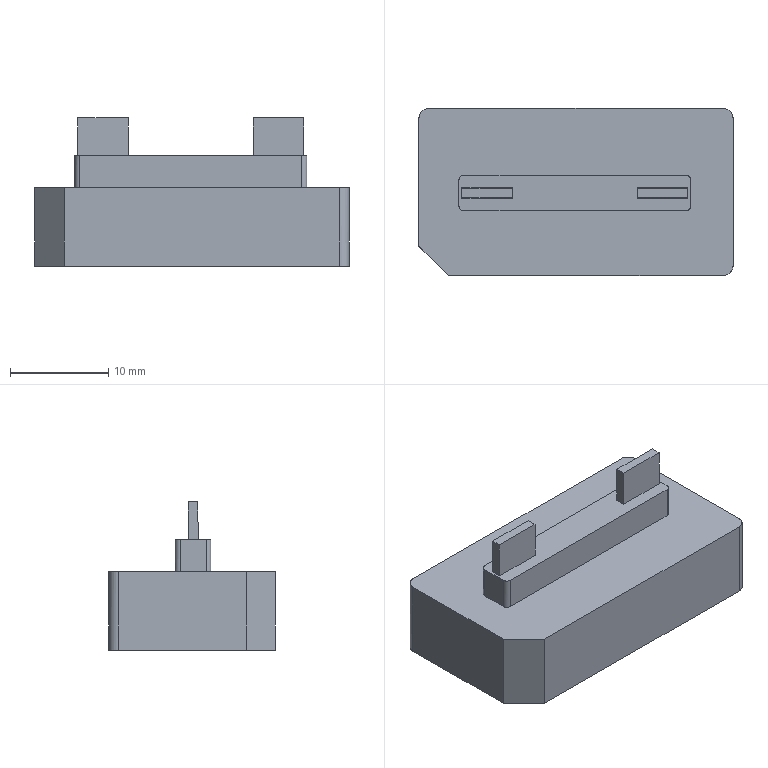NC program | PowerMill | posted by the shop | part box 32 x 17 x 15.109 mm
Lines 3100 to 3995 of 56729:
( TOOL ID   D10_1_1 )
( TOOL DIA. 10. TIP RAD 0 LENGTH 70.28 )
( Z = -4.119 )
T3 M6
T10
G91 G28 Z0
G0 G90 G54
M08
S8500 M3
X0 Y0 M8
G43 Z11.799 H3
X13.266 Y12.165
Z-2.919
G1 Z-4.119 F360
X12.287 Y6.982 F600
X9.889 Y5.783
X11.383
X11.664 Y5.776
G2 X12.775 Y5.6 I-.312 J-5.563
G1 X13.045 Y5.52
X13.311 Y5.426
G2 X14.073 Y5.062 I-2.083 J-5.347
X14.545 Y4.755 I-3.25 J-5.522
G1 X14.768 Y4.584
X14.983 Y4.401
X15.187 Y4.207
X15.381 Y4.003
G2 X15.735 Y3.565 I-4.735 J-4.197
G1 X15.895 Y3.333
X16.042 Y3.093
X16.176 Y2.845
X16.297 Y2.591
X16.405 Y2.331
X16.499 Y2.065
X16.579 Y1.795
X16.645 Y1.521
X16.696 Y1.245
X16.733 Y.965
X16.755 Y.684
X16.763 Y.403
Y-.627
X16.755 Y-.909
X16.733 Y-1.189
X16.696 Y-1.469
X16.645 Y-1.746
X16.579 Y-2.019
X16.499 Y-2.29
X16.405 Y-2.555
X16.297 Y-2.815
X16.176 Y-3.07
X16.042 Y-3.317
G2 X15.735 Y-3.789 I-5.478 J3.222
X15.381 Y-4.227 I-5.136 J3.797
G1 X15.187 Y-4.431
X14.983 Y-4.625
X14.768 Y-4.808
G2 X14.313 Y-5.139 I-3.867 J4.843
X13.825 Y-5.421 I-3.471 J5.449
X13.311 Y-5.65 I-2.868 J5.75
X12.775 Y-5.824 I-2.247 J6.004
X12.224 Y-5.941 I-1.618 J6.257
X11.664 Y-6. I-.95 J6.341
G1 X11.383 Y-6.007
X6.223
X6.042 Y-6.003
X5.661 Y-5.978
G2 X4.56 Y-5.744 I.603 J5.54
G1 X4.294 Y-5.649
X4.035 Y-5.542
G2 X3.293 Y-5.139 I2.352 J5.216
X2.837 Y-4.808 I3.524 J5.329
G1 X2.623 Y-4.625
X2.419 Y-4.431
X2.225 Y-4.227
X2.042 Y-4.013
X1.871 Y-3.789
X1.712 Y-3.558
X1.564 Y-3.317
X1.429 Y-3.07
X1.308 Y-2.815
X1.2 Y-2.555
X1.106 Y-2.29
X1.026 Y-2.019
X.961 Y-1.746
X.909 Y-1.469
X.872 Y-1.189
X.85 Y-.909
X.843 Y-.627
Y.403
X.85 Y.684
X.872 Y.965
X.909 Y1.245
X.961 Y1.521
X1.026 Y1.795
X1.106 Y2.065
X1.2 Y2.331
X1.308 Y2.591
X1.429 Y2.845
X1.564 Y3.093
X1.712 Y3.335
X1.871 Y3.565
G2 X2.196 Y3.969 I4.542 J-3.328
G1 X2.419 Y4.207
X2.623 Y4.401
G2 X3.061 Y4.755 I4.088 J-4.601
X3.533 Y5.062 I3.742 J-5.244
X4.035 Y5.318 I3.159 J-5.579
G1 X4.294 Y5.425
X4.56 Y5.52
G2 X5.104 Y5.665 I1.94 J-6.152
X5.661 Y5.753 I1.281 J-6.288
G1 X5.941 Y5.776
X6.223 Y5.783
X9.889
G0 Z5.801
G1 X3.045 Y4.743 F10000
G0 Z-4.019
G1 X2.838 Y4.583 Z-4.023 F360
X2.623 Y4.401 Z-4.028
X2.419 Y4.207 Z-4.033
X2.225 Y4.003 Z-4.038
X2.196 Y3.969 Z-4.039
X2.029 Y3.771 Z-4.043
X1.871 Y3.565 Z-4.048
X1.762 Y3.407 Z-4.051
X1.667 Y3.261 Z-4.054
X1.564 Y3.093 Z-4.058
X1.513 Y2.999 Z-4.06
X1.429 Y2.845 Z-4.063
X1.321 Y2.618 Z-4.067
X1.308 Y2.591 Z-4.068
X1.2 Y2.331 Z-4.073
X1.106 Y2.065 Z-4.077
X1.099 Y2.04 Z-4.078
X1.026 Y1.795 Z-4.082
X.974 Y1.576 Z-4.086
X.961 Y1.521 Z-4.087
X.909 Y1.245 Z-4.092
X.881 Y1.03 Z-4.096
X.872 Y.965 Z-4.097
X.85 Y.684 Z-4.102
X.843 Y.403 Z-4.107
Y.08 Z-4.113
Y-.277 Z-4.119
X-1.346 Y2.065 F600
X-1.266 Y1.795
X-1.201 Y1.521
X-1.149 Y1.245
X-1.112 Y.965
X-1.09 Y.684
X-1.083 Y.403
Y-.627
X-1.09 Y-.909
X-1.112 Y-1.189
X-1.149 Y-1.469
X-1.201 Y-1.746
X-1.266 Y-2.02
X-1.346 Y-2.29
X-1.44 Y-2.555
X-1.548 Y-2.815
X-1.669 Y-3.07
X-1.804 Y-3.317
X-1.951 Y-3.557
X-2.111 Y-3.789
X-2.282 Y-4.013
X-2.465 Y-4.227
X-2.659 Y-4.431
X-2.863 Y-4.625
X-3.077 Y-4.808
X-3.301 Y-4.98
X-3.533 Y-5.139
X-3.773 Y-5.286
X-4.021 Y-5.421
X-4.275 Y-5.542
X-4.535 Y-5.65
G2 X-5.084 Y-5.827 I-2.123 J5.636
G1 X-5.344 Y-5.889
G2 X-5.901 Y-5.978 I-1.284 J6.308
G1 X-6.181 Y-6.
X-6.463 Y-6.007
X-11.623
X-11.904 Y-6.
X-12.185 Y-5.978
X-12.464 Y-5.941
X-12.741 Y-5.889
X-13.015 Y-5.824
X-13.285 Y-5.744
X-13.551 Y-5.65
X-13.811 Y-5.542
X-14.065 Y-5.421
X-14.313 Y-5.286
X-14.553 Y-5.139
X-14.785 Y-4.98
X-15.008 Y-4.808
X-15.223 Y-4.625
X-15.427 Y-4.431
X-15.621 Y-4.227
X-15.804 Y-4.013
X-15.975 Y-3.789
X-16.135 Y-3.557
X-16.282 Y-3.317
X-16.416 Y-3.07
X-16.537 Y-2.815
X-16.645 Y-2.555
X-16.739 Y-2.29
X-16.819 Y-2.019
X-16.885 Y-1.746
X-16.936 Y-1.469
X-16.973 Y-1.189
X-16.995 Y-.909
X-17.003 Y-.627
Y.403
X-16.995 Y.684
G2 X-16.936 Y1.245 I6.275 J-.376
G1 X-16.885 Y1.521
X-16.819 Y1.795
X-16.739 Y2.065
X-16.645 Y2.331
X-16.537 Y2.591
X-16.416 Y2.845
X-16.282 Y3.093
X-16.135 Y3.333
G2 X-15.804 Y3.789 I5.175 J-3.412
X-15.427 Y4.207 I4.982 J-4.107
X-15.008 Y4.584 I4.337 J-4.396
G1 X-14.785 Y4.755
X-14.553 Y4.915
G2 X-14.065 Y5.197 I3.397 J-5.321
X-13.551 Y5.426 I2.892 J-5.803
X-13.015 Y5.6 I2.266 J-6.062
X-12.464 Y5.717 I1.621 J-6.272
X-11.904 Y5.776 I.957 J-6.414
G1 X-11.623 Y5.783
X-6.463
X-6.12 Y5.771
X-5.901 Y5.753
G2 X-5.344 Y5.665 I-.726 J-6.38
X-4.801 Y5.52 I-1.395 J-6.294
G1 X-4.534 Y5.425
X-4.275 Y5.318
G2 X-3.533 Y4.915 I-2.362 J-5.234
X-3.077 Y4.584 I-3.539 J-5.349
G1 X-2.863 Y4.401
X-2.659 Y4.207
X-2.465 Y4.003
X-2.282 Y3.789
G2 X-1.951 Y3.333 I-4.962 J-3.953
G1 X-1.804 Y3.093
X-1.669 Y2.845
X-1.548 Y2.591
X-1.44 Y2.331
X-1.346 Y2.065
G0 Z3.999
G1 X-7.413 Y11.029 F10000
G0 Z.929
G1 Z-.271 F360
Y5.754 F600
X-7.424 Y1.208
X-10.182 Y1.215
G3 X-11.368 Y-.08 I-.003 J-1.188
G1 X-11.343 Y-.362
G3 X-9.767 Y-1.377 I1.183 J.106
G1 X-7.143 Y-.459
G3 X-7.424 Y1.208 I-.283 J.809
G1 X-7.413 Y5.754
G0 Z3.999
G1 X7.324 Y-11.253 F10000
G0 Z.929
G1 Z-.271 F360
Y-5.978 F600
X7.252 Y-1.524
X9.902 Y-1.481
G3 X11.073 Y-.311 I-.019 J1.19
G1 X11.08 Y.105
G3 X9.764 Y1.308 I-1.19 J.02
G1 X7.066 Y1.02
G3 X6.333 Y.232 I.087 J-.816
G1 X6.307 Y-.563
G3 X7.252 Y-1.524 I.93 J-.031
G1 X7.324 Y-5.978
G0 Z11.799
X0 Y0
Z9.799
X-21.36 Y-15.215
Z-6.11
G1 Z-7.31 F360
X-17.631 Y-11.485 F600
X-9.275 Y-7.307
X-11.423
G2 X-12.383 Y-7.228 I.037 J6.331
G1 X-12.603 Y-7.187
G2 X-13.354 Y-6.981 I1.378 J6.492
G1 X-13.574 Y-6.899
G2 X-14.09 Y-6.667 I2.79 J6.895
G1 X-14.303 Y-6.553
G2 X-14.79 Y-6.245 I3.027 J5.321
G1 X-14.99 Y-6.101
G2 X-15.414 Y-5.743 I3.291 J4.325
X-15.943 Y-5.187 I4.292 J4.622
X-16.663 Y-4.094 I4.738 J3.9
G1 X-16.767 Y-3.875
G2 X-16.976 Y-3.358 I5.726 J2.624
G1 X-17.049 Y-3.135
X-17.12 Y-2.873
X-17.182 Y-2.608
X-17.224 Y-2.388
X-17.256 Y-2.166
G2 X-17.303 Y-1.427 I6.597 J.79
G1 Y1.203
G2 X-17.224 Y2.164 I6.347 J-.038
G1 X-17.182 Y2.384
G2 X-16.976 Y3.134 I6.449 J-1.366
G1 X-16.895 Y3.354
X-16.767 Y3.651
G2 X-16.39 Y4.345 I4.892 J-2.203
X-15.782 Y5.149 I5.021 J-3.173
X-15.368 Y5.562 I5.712 J-5.299
G1 X-15.183 Y5.724
G2 X-14.303 Y6.329 I4.042 J-4.931
G1 X-14.09 Y6.443
G2 X-13.354 Y6.757 I2.977 J-5.959
X-12.383 Y7.004 I2.05 J-6.019
G1 X-12.162 Y7.036
G2 X-11.423 Y7.083 I.786 J-6.524
G1 X11.183
G2 X12.363 Y6.963 I-.025 J-6.106
G1 X12.742 Y6.871
X12.89 Y6.829
X13.114 Y6.757
G2 X14.063 Y6.329 I-2.115 J-5.961
X14.55 Y6.021 I-3.069 J-5.386
G1 X14.75 Y5.877
X14.942 Y5.724
G2 X15.306 Y5.392 I-3.861 J-4.597
X15.703 Y4.963 I-4.553 J-4.612
X16.423 Y3.87 I-4.747 J-3.906
X16.655 Y3.354 I-6.686 J-3.317
G1 X16.736 Y3.134
X16.809 Y2.911
G2 X16.984 Y2.164 I-6.458 J-1.906
X17.063 Y1.203 I-6.305 J-1.002
G1 X17.061 Y-1.524
G2 X16.942 Y-2.608 I-5.945 J.1
G1 X16.88 Y-2.873
X16.809 Y-3.135
X16.736 Y-3.358
X16.655 Y-3.578
G2 X16.423 Y-4.094 I-6.913 J2.799
G1 X16.309 Y-4.308
X16.185 Y-4.516
G2 X15.857 Y-4.994 I-6.278 J3.967
G1 X15.703 Y-5.187
G2 X15.371 Y-5.551 I-4.612 J3.874
X14.942 Y-5.948 I-4.427 J4.353
G1 X14.75 Y-6.101
G2 X14.272 Y-6.43 I-4.572 J6.136
G1 X14.063 Y-6.553
X13.85 Y-6.667
X13.631 Y-6.771
X13.334 Y-6.899
X13.114 Y-6.981
G2 X12.143 Y-7.228 I-2.055 J6.042
G1 X11.922 Y-7.26
X11.661 Y-7.286
X11.401 Y-7.303
X11.183 Y-7.307
X-9.275
G0 Z9.799
Z10.799
X0 Y0
X15.022 Y-6.093
Z-6.08
G1 Z-7.28 F360
G3 X13.883 Y-6.23 I-.405 J-1.444 F600
G2 X11.136 Y-6.937 I-2.702 J4.804
G1 X5.519
X-.091
X-11.504 Y-6.936
G2 X-16.932 Y-1.46 I.083 J5.511
G1 Y1.281
G2 X-11.501 Y6.712 I5.511 J-.079
G1 X11.137 Y6.713
G2 X16.692 Y1.278 I.044 J-5.512
G1 Y-1.462
G2 X13.883 Y-6.23 I-5.512 J.037
G3 X13.174 Y-7.132 I.735 J-1.307
G1 X14.932 Y-6.065
G3 X13.791 Y-6.189 I-.421 J-1.44
G2 X11.136 Y-6.857 I-2.61 J4.764
G1 X5.519
X-.091
X-11.501 Y-6.856
G2 X-16.852 Y-1.46 I.08 J5.431
G1 Y1.278
G2 X-11.501 Y6.632 I5.431 J-.076
G1 X11.136 Y6.633
G2 X16.612 Y1.278 I.045 J-5.432
G1 Y-1.46
G2 X13.791 Y-6.189 I-5.432 J.035
G3 X13.072 Y-7.084 I.721 J-1.315
G0 Z10.799
X0 Y0
Z9.799
X21.337 Y-16.587
Z-14.01
G1 Z-15.21 F360
G3 X18.475 Y-12.487 I-1.431 J2.05 F600
G1 X18.382 Y-12.551
X18.381 Y-12.552
X18.379 Y-12.553
X18.128 Y-12.713
X18.126 Y-12.715
X18.124 Y-12.716
X17.743 Y-12.926
X17.74 Y-12.927
X17.738 Y-12.928
X17.422 Y-13.077
X17.42 Y-13.078
X17.418 Y-13.079
X17.102 Y-13.205
X17.1 Y-13.206
X17.097 Y-13.207
X16.781 Y-13.313
X16.78 Y-13.314
X16.778
X16.639 Y-13.355
X16.638
X16.637
X16.46 Y-13.402
X16.458
X16.457 Y-13.403
X16.14 Y-13.472
X16.138
X16.136 Y-13.473
X15.82 Y-13.524
X15.818 Y-13.525
X15.816
X15.5 Y-13.559
X15.498
X15.496
X15.179 Y-13.577
X15.178
X15.176
X14.86 Y-13.58
X14.859
X-12.962
X-12.963
X-12.964
X-13.28 Y-13.572
X-13.283
X-13.285
X-13.601 Y-13.544
X-13.604
X-13.606
X-13.922 Y-13.496
X-13.925 Y-13.495
X-13.928
X-14.244 Y-13.425
X-14.246
X-14.248 Y-13.424
X-14.495 Y-13.355
X-14.497 Y-13.354
X-14.5
X-14.886 Y-13.217
X-14.888 Y-13.216
X-14.891 Y-13.215
X-15.207 Y-13.075
X-15.21 Y-13.074
X-15.212 Y-13.073
X-15.528 Y-12.906
X-15.531 Y-12.905
X-15.533 Y-12.903
X-15.837 Y-12.714
X-15.84 Y-12.712
X-15.842 Y-12.71
X-16.171 Y-12.469
X-16.172 Y-12.468
X-16.174 Y-12.466
X-16.265 Y-12.392
X-16.267 Y-12.39
X-16.268 Y-12.389
X-16.493 Y-12.189
X-16.494 Y-12.187
X-16.496 Y-12.186
X-16.613 Y-12.071
X-16.614 Y-12.07
X-19.658 Y-9.025
X-19.659 Y-9.024
X-19.66 Y-9.023
X-19.768 Y-8.907
X-19.77 Y-8.905
X-19.771 Y-8.904
X-19.978 Y-8.659
X-19.979 Y-8.658
X-19.98 Y-8.657
X-20.036 Y-8.585
X-20.037 Y-8.584
X-20.038 Y-8.582
X-20.261 Y-8.266
X-20.263 Y-8.263
X-20.264 Y-8.261
X-20.453 Y-7.945
X-20.454 Y-7.942
X-20.456 Y-7.94
X-20.615 Y-7.623
X-20.616 Y-7.621
X-20.617 Y-7.618
X-20.75 Y-7.302
X-20.751 Y-7.3
Y-7.297
X-20.859 Y-6.981
X-20.86 Y-6.979
X-20.861 Y-6.976
X-20.943 Y-6.672
Y-6.67
X-20.944 Y-6.667
X-21.01 Y-6.339
X-21.011 Y-6.336
Y-6.334
X-21.054 Y-6.017
Y-6.015
Y-6.012
X-21.076 Y-5.696
Y-5.694
Y-5.692
X-21.08 Y-5.375
Y-5.374
X-21.079 Y7.588
Y7.589
Y7.591
X-21.066 Y7.907
Y7.909
Y7.911
X-21.036 Y8.227
Y8.229
Y8.231
X-20.989 Y8.548
Y8.549
X-20.988 Y8.551
X-20.944 Y8.778
Y8.78
X-20.943 Y8.782
X-20.841 Y9.188
X-20.84 Y9.19
Y9.193
X-20.738 Y9.509
Y9.511
X-20.737 Y9.513
X-20.624 Y9.81
X-20.623 Y9.812
X-20.622 Y9.814
X-20.472 Y10.149
X-20.471 Y10.152
X-20.47 Y10.154
X-20.305 Y10.47
X-20.304 Y10.472
X-20.303 Y10.474
X-20.113 Y10.79
X-20.112 Y10.792
X-20.11 Y10.793
X-19.984 Y10.983
X-19.983 Y10.984
X-19.982 Y10.985
X-19.891 Y11.112
X-19.89 Y11.113
X-19.889 Y11.115
X-19.664 Y11.401
X-19.662 Y11.403
X-19.66 Y11.405
X-19.347 Y11.751
X-19.345 Y11.753
X-19.342 Y11.755
X-19.024 Y12.058
X-19.022 Y12.06
X-19.02 Y12.062
X-18.703 Y12.322
X-18.702 Y12.323
X-18.701 Y12.324
X-18.608 Y12.394
X-18.607
X-18.606 Y12.395
X-18.382 Y12.551
X-18.381 Y12.552
X-18.379 Y12.553
X-18.128 Y12.713
X-18.126 Y12.715
X-18.124 Y12.716
X-17.743 Y12.926
X-17.74 Y12.927
X-17.738 Y12.928
X-17.422 Y13.077
X-17.42 Y13.078
X-17.418 Y13.079
X-17.102 Y13.205
X-17.1 Y13.206
X-17.097 Y13.207
X-16.781 Y13.313
X-16.779 Y13.314
X-16.777
X-16.461 Y13.402
X-16.459
X-16.457 Y13.403
X-16.14 Y13.472
X-16.138
X-16.136 Y13.473
X-15.82 Y13.524
X-15.818 Y13.525
X-15.816
X-15.5 Y13.559
X-15.498
X-15.496
X-15.179 Y13.577
X-15.178
X-15.176
X-14.86 Y13.58
X-14.859
X0
X14.859
X14.86
X15.176 Y13.577
X15.178
X15.179
X15.495 Y13.56
X15.498
X15.5 Y13.559
X15.816 Y13.525
X15.818
X15.82 Y13.524
X16.136 Y13.473
X16.138 Y13.472
X16.141
X16.457 Y13.403
X16.459 Y13.402
X16.461
X16.777 Y13.314
X16.779
X16.781 Y13.313
X17.098 Y13.206
X17.1 Y13.205
X17.101
X17.418 Y13.079
X17.42 Y13.078
X17.422 Y13.077
X17.738 Y12.928
X17.74 Y12.927
X17.742 Y12.926
X18.058 Y12.755
X18.061 Y12.754
X18.063 Y12.752
X18.379 Y12.555
X18.381 Y12.553
X18.382 Y12.552
X18.606 Y12.395
X18.607 Y12.394
X18.608
X18.701 Y12.324
X18.702 Y12.323
X18.703 Y12.322
X19.004 Y12.075
X19.006 Y12.074
X19.008 Y12.072
X19.34 Y11.758
X19.342 Y11.756
X19.344 Y11.754
X19.634 Y11.435
X19.636 Y11.433
X19.638 Y11.431
X19.889 Y11.115
X19.89 Y11.113
X19.891 Y11.112
X19.982 Y10.985
X19.983 Y10.983
X19.984 Y10.982
X20.11 Y10.794
X20.111 Y10.792
X20.112 Y10.79
X20.302 Y10.476
X20.303 Y10.474
X20.304 Y10.472
X20.47 Y10.154
X20.471 Y10.152
X20.472 Y10.149
X20.614 Y9.833
X20.615 Y9.831
X20.616 Y9.829
X20.737 Y9.513
X20.738 Y9.511
X20.739 Y9.509
X20.84 Y9.193
Y9.19
X20.841 Y9.188
X20.923 Y8.872
X20.924 Y8.87
Y8.868
X20.988 Y8.552
Y8.55
Y8.548
X21.036 Y8.232
Y8.229
Y8.227
X21.065 Y7.911
Y7.909
X21.066 Y7.907
X21.079 Y7.591
Y7.589
Y7.587
Y-7.587
Y-7.589
Y-7.591
X21.066 Y-7.907
Y-7.909
Y-7.911
X21.036 Y-8.227
Y-8.229
Y-8.231
X20.989 Y-8.548
Y-8.549
X20.988 Y-8.551
X20.944 Y-8.778
Y-8.78
X20.943 Y-8.782
X20.841 Y-9.188
X20.84 Y-9.19
Y-9.193
X20.738 Y-9.509
Y-9.511
X20.737 Y-9.513
X20.624 Y-9.81
X20.623 Y-9.812
X20.622 Y-9.814
X20.472 Y-10.149
X20.471 Y-10.152
X20.47 Y-10.154
X20.305 Y-10.47
X20.304 Y-10.472
X20.303 Y-10.474
X20.113 Y-10.79
X20.112 Y-10.792
X20.11 Y-10.793
X19.984 Y-10.983
X19.983 Y-10.984
X19.982 Y-10.985
X19.891 Y-11.112
X19.89 Y-11.113
X19.889 Y-11.115
X19.664 Y-11.401
X19.662 Y-11.403
X19.66 Y-11.405
X19.347 Y-11.751
X19.345 Y-11.753
X19.342 Y-11.755
X19.024 Y-12.058
X19.022 Y-12.06
X19.02 Y-12.062
X18.703 Y-12.322
X18.702 Y-12.323
X18.701 Y-12.324
X18.608 Y-12.394
X18.607
X18.606 Y-12.395
X18.475 Y-12.487
G3 X21.337 Y-16.587 I1.431 J-2.05
G1 X21.285 Y-16.525
G3 X18.424 Y-12.425 I-1.431 J2.05
G1 X18.336 Y-12.486
X18.085 Y-12.646
X17.704 Y-12.856
X17.388 Y-13.004
X17.072 Y-13.131
X16.756 Y-13.237
X16.616 Y-13.278
X16.44 Y-13.325
X16.123 Y-13.394
X15.807 Y-13.445
X15.491 Y-13.48
X15.175 Y-13.497
X14.859 Y-13.5
X-12.962
X-13.278 Y-13.492
X-13.594 Y-13.465
X-13.91 Y-13.416
X-14.227 Y-13.347
X-14.473 Y-13.278
X-14.859 Y-13.142
X-15.175 Y-13.002
X-15.491 Y-12.835
X-15.795 Y-12.646
X-16.123 Y-12.404
X-16.215 Y-12.33
X-16.44 Y-12.129
X-16.558 Y-12.014
X-19.285 Y-9.286
X-19.601 Y-8.969
X-19.71 Y-8.852
X-19.917 Y-8.607
X-19.973 Y-8.536
X-20.196 Y-8.22
X-20.384 Y-7.904
X-20.543 Y-7.587
X-20.676 Y-7.271
X-20.784 Y-6.955
X-20.866 Y-6.651
X-20.932 Y-6.323
X-20.974 Y-6.007
X-20.996 Y-5.691
X-21. Y-5.374
Y7.271
X-20.999 Y7.587
X-20.986 Y7.904
X-20.957 Y8.22
X-20.91 Y8.536
X-20.866 Y8.763
X-20.763 Y9.168
X-20.662 Y9.484
X-20.549 Y9.781
X-20.399 Y10.117
X-20.234 Y10.433
X-20.044 Y10.749
X-19.917 Y10.938
X-19.826 Y11.065
X-19.601 Y11.351
X-19.287 Y11.697
X-18.969 Y12.
X-18.653 Y12.26
X-18.56 Y12.33
X-18.336 Y12.486
X-18.085 Y12.646
X-17.704 Y12.856
X-17.388 Y13.004
X-17.072 Y13.131
X-16.756 Y13.237
X-16.44 Y13.325
X-16.123 Y13.394
X-15.807 Y13.445
X-15.491 Y13.48
X-15.175 Y13.497
X-14.859 Y13.5
X0
X14.859
X15.175 Y13.497
X15.491 Y13.48
X15.807 Y13.445
X16.123 Y13.394
X16.44 Y13.325
X16.756 Y13.237
X17.072 Y13.13
X17.388 Y13.004
X17.704 Y12.855
X18.02 Y12.684
X18.336 Y12.487
X18.56 Y12.33
X18.653 Y12.26
X18.953 Y12.014
X19.285 Y11.7
X19.575 Y11.381
X19.826 Y11.065
X19.917 Y10.938
X20.044 Y10.749
X20.233 Y10.434
X20.399 Y10.117
X20.541 Y9.801
X20.662 Y9.484
X20.763 Y9.168
X20.846 Y8.852
X20.909 Y8.536
X20.957 Y8.22
X20.986 Y7.904
X20.999 Y7.587
X21. Y7.271
Y-7.271
X20.999 Y-7.587
X20.986 Y-7.904
X20.957 Y-8.22
X20.91 Y-8.536
X20.866 Y-8.763
X20.763 Y-9.168
X20.662 Y-9.484
X20.549 Y-9.781
X20.399 Y-10.117
X20.234 Y-10.433
X20.044 Y-10.749
X19.917 Y-10.938
X19.826 Y-11.065
X19.601 Y-11.351
X19.287 Y-11.697
X18.969 Y-12.
X18.653 Y-12.26
X18.56 Y-12.33
X18.424 Y-12.425
G3 X21.285 Y-16.525 I1.431 J-2.05
G0 Z9.799
Z10.799
X0 Y0
M9
M5
M01